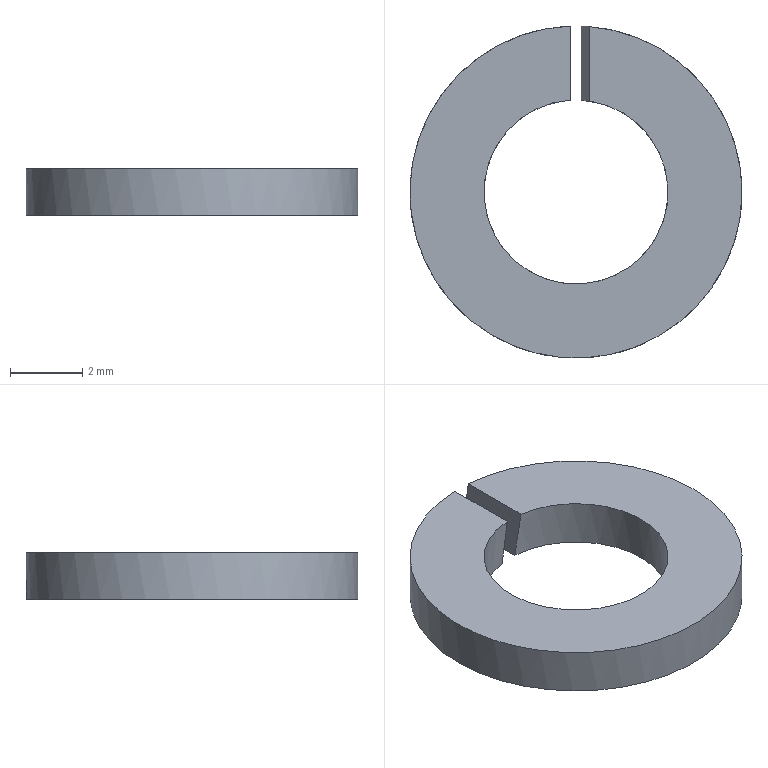Part | NX | features 5003_309_SLW5 2 | 1 solid | 6 faces | box 9.2 x 9.198 x 1.3 mm | volume 58.475 mm3 | plane 4 | cylinder 2 | commonest cylinder face diameters 5.1 x1 9.2 x1
STEP:
#1=CARTESIAN_POINT('',(188.375,-167.402,-182.7));
#2=VERTEX_POINT('',#1);
#3=CARTESIAN_POINT('',(188.375,-169.454,-182.7));
#4=VERTEX_POINT('',#3);
#5=CARTESIAN_POINT('',(188.375,-167.4,-182.7));
#6=DIRECTION('',(0.,-1.,0.));
#7=VECTOR('',#6,1000.);
#8=LINE('',#5,#7);
#9=EDGE_CURVE('',#2,#4,#8,.T.);
#10=ORIENTED_EDGE('',*,*,#9,.F.);
#11=CARTESIAN_POINT('',(188.895,-167.415,-182.7));
#12=VERTEX_POINT('',#11);
#13=CARTESIAN_POINT('',(188.525,-172.,-182.7));
#14=DIRECTION('',(0.,0.,1.));
#15=DIRECTION('',(0.,1.,0.));
#16=AXIS2_PLACEMENT_3D('',#13,#14,#15);
#17=CIRCLE('',#16,4.6);
#18=EDGE_CURVE('',#2,#12,#17,.T.);
#19=ORIENTED_EDGE('',*,*,#18,.T.);
#20=CARTESIAN_POINT('',(188.895,-169.477,-182.7));
#21=VERTEX_POINT('',#20);
#22=CARTESIAN_POINT('',(188.895,-167.4,-182.7));
#23=DIRECTION('',(0.,-1.,0.));
#24=VECTOR('',#23,1000.);
#25=LINE('',#22,#24);
#26=EDGE_CURVE('',#12,#21,#25,.T.);
#27=ORIENTED_EDGE('',*,*,#26,.T.);
#28=CARTESIAN_POINT('',(188.525,-172.,-182.7));
#29=DIRECTION('',(0.,0.,1.));
#30=DIRECTION('',(0.,1.,0.));
#31=AXIS2_PLACEMENT_3D('',#28,#29,#30);
#32=CIRCLE('',#31,2.55);
#33=EDGE_CURVE('',#4,#21,#32,.T.);
#34=ORIENTED_EDGE('',*,*,#33,.F.);
#35=EDGE_LOOP('',(#10,#19,#27,#34));
#36=FACE_BOUND('',#35,.T.);
#37=CARTESIAN_POINT('',(185.975,-172.,-182.7));
#38=DIRECTION('',(0.,0.,-1.));
#39=DIRECTION('',(0.,-1.,0.));
#40=AXIS2_PLACEMENT_3D('',#37,#38,#39);
#41=PLANE('',#40);
#42=ADVANCED_FACE('',(#36),#41,.F.);
#43=CARTESIAN_POINT('',(188.155,-167.415,-184.));
#44=VERTEX_POINT('',#43);
#45=CARTESIAN_POINT('',(188.525,-172.,-181.814));
#46=DIRECTION('',(0.986,0.,-0.1669));
#47=DIRECTION('',(0.1669,0.,0.986));
#48=AXIS2_PLACEMENT_3D('',#45,#46,#47);
#49=ELLIPSE('',#48,27.568,4.6);
#50=EDGE_CURVE('',#44,#2,#49,.T.);
#51=ORIENTED_EDGE('',*,*,#50,.F.);
#52=CARTESIAN_POINT('',(188.675,-167.402,-184.));
#53=VERTEX_POINT('',#52);
#54=CARTESIAN_POINT('',(188.525,-172.,-184.));
#55=DIRECTION('',(0.,0.,1.));
#56=DIRECTION('',(0.,1.,0.));
#57=AXIS2_PLACEMENT_3D('',#54,#55,#56);
#58=CIRCLE('',#57,4.6);
#59=EDGE_CURVE('',#44,#53,#58,.T.);
#60=ORIENTED_EDGE('',*,*,#59,.T.);
#61=CARTESIAN_POINT('',(188.525,-172.,-184.886));
#62=DIRECTION('',(-0.986,0.,0.1669));
#63=DIRECTION('',(0.1669,0.,0.986));
#64=AXIS2_PLACEMENT_3D('',#61,#62,#63);
#65=ELLIPSE('',#64,27.568,4.6);
#66=EDGE_CURVE('',#12,#53,#65,.T.);
#67=ORIENTED_EDGE('',*,*,#66,.F.);
#68=ORIENTED_EDGE('',*,*,#18,.F.);
#69=EDGE_LOOP('',(#51,#60,#67,#68));
#70=FACE_BOUND('',#69,.T.);
#71=CARTESIAN_POINT('',(188.525,-172.,-182.7));
#72=DIRECTION('',(0.,0.,1.));
#73=DIRECTION('',(0.,1.,0.));
#74=AXIS2_PLACEMENT_3D('',#71,#72,#73);
#75=CYLINDRICAL_SURFACE('',#74,4.6);
#76=ADVANCED_FACE('',(#70),#75,.T.);
#77=CARTESIAN_POINT('',(188.155,-169.477,-184.));
#78=VERTEX_POINT('',#77);
#79=CARTESIAN_POINT('',(188.155,-167.4,-184.));
#80=DIRECTION('',(0.,-1.,0.));
#81=VECTOR('',#80,1000.);
#82=LINE('',#79,#81);
#83=EDGE_CURVE('',#44,#78,#82,.T.);
#84=ORIENTED_EDGE('',*,*,#83,.T.);
#85=CARTESIAN_POINT('',(188.675,-169.454,-184.));
#86=VERTEX_POINT('',#85);
#87=CARTESIAN_POINT('',(188.525,-172.,-184.));
#88=DIRECTION('',(0.,0.,1.));
#89=DIRECTION('',(0.,1.,0.));
#90=AXIS2_PLACEMENT_3D('',#87,#88,#89);
#91=CIRCLE('',#90,2.55);
#92=EDGE_CURVE('',#78,#86,#91,.T.);
#93=ORIENTED_EDGE('',*,*,#92,.T.);
#94=CARTESIAN_POINT('',(188.675,-167.4,-184.));
#95=DIRECTION('',(0.,-1.,0.));
#96=VECTOR('',#95,1000.);
#97=LINE('',#94,#96);
#98=EDGE_CURVE('',#53,#86,#97,.T.);
#99=ORIENTED_EDGE('',*,*,#98,.F.);
#100=ORIENTED_EDGE('',*,*,#59,.F.);
#101=EDGE_LOOP('',(#84,#93,#99,#100));
#102=FACE_BOUND('',#101,.T.);
#103=CARTESIAN_POINT('',(185.975,-172.,-184.));
#104=DIRECTION('',(0.,0.,1.));
#105=DIRECTION('',(0.,1.,0.));
#106=AXIS2_PLACEMENT_3D('',#103,#104,#105);
#107=PLANE('',#106);
#108=ADVANCED_FACE('',(#102),#107,.F.);
#109=CARTESIAN_POINT('',(188.525,-172.,-181.814));
#110=DIRECTION('',(0.986,0.,-0.1669));
#111=DIRECTION('',(0.1669,0.,0.986));
#112=AXIS2_PLACEMENT_3D('',#109,#110,#111);
#113=ELLIPSE('',#112,15.282,2.55);
#114=EDGE_CURVE('',#4,#78,#113,.F.);
#115=ORIENTED_EDGE('',*,*,#114,.F.);
#116=ORIENTED_EDGE('',*,*,#33,.T.);
#117=CARTESIAN_POINT('',(188.525,-172.,-184.886));
#118=DIRECTION('',(-0.986,0.,0.1669));
#119=DIRECTION('',(0.1669,0.,0.986));
#120=AXIS2_PLACEMENT_3D('',#117,#118,#119);
#121=ELLIPSE('',#120,15.282,2.55);
#122=EDGE_CURVE('',#86,#21,#121,.F.);
#123=ORIENTED_EDGE('',*,*,#122,.F.);
#124=ORIENTED_EDGE('',*,*,#92,.F.);
#125=EDGE_LOOP('',(#115,#116,#123,#124));
#126=FACE_BOUND('',#125,.T.);
#127=CARTESIAN_POINT('',(188.525,-172.,-182.7));
#128=DIRECTION('',(0.,0.,1.));
#129=DIRECTION('',(0.,1.,0.));
#130=AXIS2_PLACEMENT_3D('',#127,#128,#129);
#131=CYLINDRICAL_SURFACE('',#130,2.55);
#132=ADVANCED_FACE('',(#126),#131,.F.);
#133=ORIENTED_EDGE('',*,*,#66,.T.);
#134=ORIENTED_EDGE('',*,*,#98,.T.);
#135=ORIENTED_EDGE('',*,*,#122,.T.);
#136=ORIENTED_EDGE('',*,*,#26,.F.);
#137=EDGE_LOOP('',(#133,#134,#135,#136));
#138=FACE_BOUND('',#137,.T.);
#139=CARTESIAN_POINT('',(188.895,-167.4,-182.7));
#140=DIRECTION('',(-0.986,0.,0.1669));
#141=DIRECTION('',(0.1669,0.,0.986));
#142=AXIS2_PLACEMENT_3D('',#139,#140,#141);
#143=PLANE('',#142);
#144=ADVANCED_FACE('',(#138),#143,.T.);
#145=ORIENTED_EDGE('',*,*,#50,.T.);
#146=ORIENTED_EDGE('',*,*,#9,.T.);
#147=ORIENTED_EDGE('',*,*,#114,.T.);
#148=ORIENTED_EDGE('',*,*,#83,.F.);
#149=EDGE_LOOP('',(#145,#146,#147,#148));
#150=FACE_BOUND('',#149,.T.);
#151=CARTESIAN_POINT('',(188.155,-167.4,-184.));
#152=DIRECTION('',(0.986,0.,-0.1669));
#153=DIRECTION('',(-0.1669,0.,-0.986));
#154=AXIS2_PLACEMENT_3D('',#151,#152,#153);
#155=PLANE('',#154);
#156=ADVANCED_FACE('',(#150),#155,.T.);
#157=CLOSED_SHELL('',(#42,#76,#108,#132,#144,#156));
#158=MANIFOLD_SOLID_BREP('',#157);
#159=(LENGTH_UNIT()NAMED_UNIT(*)SI_UNIT(.MILLI.,.METRE.));
#160=UNCERTAINTY_MEASURE_WITH_UNIT(LENGTH_MEASURE(0.00001),#159,'','');
#161=(NAMED_UNIT(*)PLANE_ANGLE_UNIT()SI_UNIT($,.RADIAN.));
#162=(NAMED_UNIT(*)SI_UNIT($,.STERADIAN.)SOLID_ANGLE_UNIT());
#163=(GEOMETRIC_REPRESENTATION_CONTEXT(3)GLOBAL_UNCERTAINTY_ASSIGNED_CONTEXT((#160))GLOBAL_UNIT_ASSIGNED_CONTEXT((#159,#161,#162))REPRESENTATION_CONTEXT('',''));
#164=ADVANCED_BREP_SHAPE_REPRESENTATION('',(#158),#163);